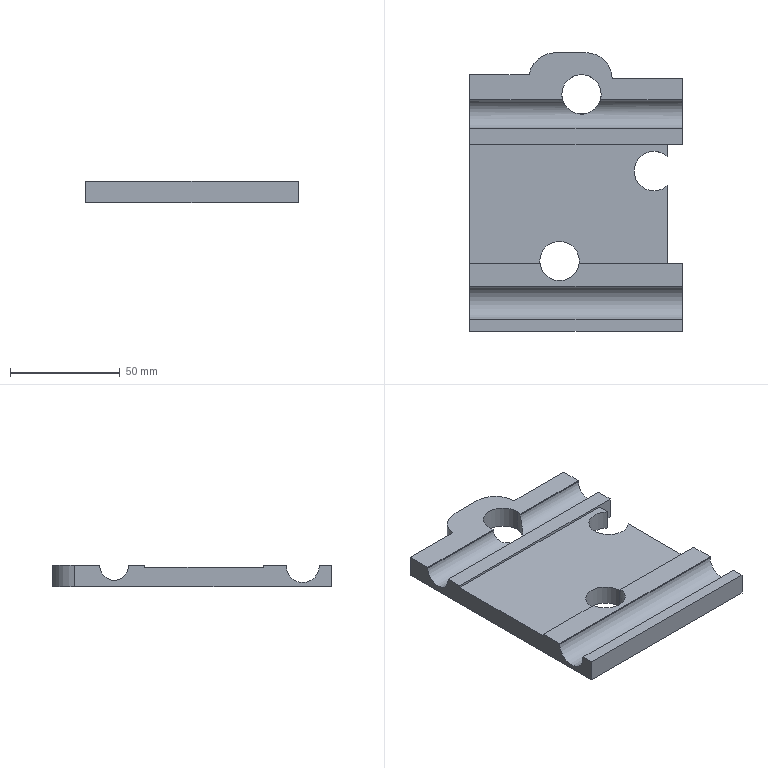Part | SolidWorks | features BaseBody 1 | 1 solid | 32 faces | box 97 x 127 x 10 mm | volume 84479 mm3 | plane 23 | cylinder 9 | commonest cylinder face diameters 18 x5 24 x2 13 x1 15 x1
STEP:
#1=CARTESIAN_POINT('',(60.,108.,10.));
#2=VERTEX_POINT('',#1);
#3=CARTESIAN_POINT('',(42.,108.,10.));
#4=VERTEX_POINT('',#3);
#5=CARTESIAN_POINT('',(51.,108.,10.));
#6=DIRECTION('',(0.,0.,1.));
#7=DIRECTION('',(1.,0.,0.));
#8=AXIS2_PLACEMENT_3D('',#5,#6,#7);
#9=CIRCLE('',#8,9.);
#10=EDGE_CURVE('',#2,#4,#9,.T.);
#11=ORIENTED_EDGE('',*,*,#10,.T.);
#12=CARTESIAN_POINT('',(42.,108.,0.));
#13=VERTEX_POINT('',#12);
#14=CARTESIAN_POINT('',(42.,108.,10.));
#15=DIRECTION('',(0.,0.,-1.));
#16=VECTOR('',#15,1000.);
#17=LINE('',#14,#16);
#18=EDGE_CURVE('',#4,#13,#17,.T.);
#19=ORIENTED_EDGE('',*,*,#18,.T.);
#20=CARTESIAN_POINT('',(60.,108.,0.));
#21=VERTEX_POINT('',#20);
#22=CARTESIAN_POINT('',(51.,108.,0.));
#23=DIRECTION('',(0.,0.,1.));
#24=DIRECTION('',(1.,0.,0.));
#25=AXIS2_PLACEMENT_3D('',#22,#23,#24);
#26=CIRCLE('',#25,9.);
#27=EDGE_CURVE('',#21,#13,#26,.T.);
#28=ORIENTED_EDGE('',*,*,#27,.F.);
#29=CARTESIAN_POINT('',(60.,108.,10.));
#30=DIRECTION('',(0.,0.,-1.));
#31=VECTOR('',#30,1000.);
#32=LINE('',#29,#31);
#33=EDGE_CURVE('',#2,#21,#32,.T.);
#34=ORIENTED_EDGE('',*,*,#33,.F.);
#35=EDGE_LOOP('',(#11,#19,#28,#34));
#36=FACE_OUTER_BOUND('',#35,.T.);
#37=CARTESIAN_POINT('',(51.,108.,10.));
#38=DIRECTION('',(0.,0.,-1.));
#39=DIRECTION('',(1.,0.,0.));
#40=AXIS2_PLACEMENT_3D('',#37,#38,#39);
#41=CYLINDRICAL_SURFACE('',#40,9.);
#42=ADVANCED_FACE('',(#36),#41,.F.);
#43=CARTESIAN_POINT('',(50.,32.,9.));
#44=VERTEX_POINT('',#43);
#45=CARTESIAN_POINT('',(32.,32.,9.));
#46=VERTEX_POINT('',#45);
#47=CARTESIAN_POINT('',(41.,32.,9.));
#48=DIRECTION('',(0.,0.,1.));
#49=DIRECTION('',(-1.,0.,0.));
#50=AXIS2_PLACEMENT_3D('',#47,#48,#49);
#51=CIRCLE('',#50,9.);
#52=EDGE_CURVE('',#44,#46,#51,.T.);
#53=ORIENTED_EDGE('',*,*,#52,.T.);
#54=CARTESIAN_POINT('',(32.,32.,0.));
#55=VERTEX_POINT('',#54);
#56=CARTESIAN_POINT('',(32.,32.,10.));
#57=DIRECTION('',(0.,0.,-1.));
#58=VECTOR('',#57,1000.);
#59=LINE('',#56,#58);
#60=EDGE_CURVE('',#46,#55,#59,.T.);
#61=ORIENTED_EDGE('',*,*,#60,.T.);
#62=CARTESIAN_POINT('',(50.,32.,0.));
#63=VERTEX_POINT('',#62);
#64=CARTESIAN_POINT('',(41.,32.,0.));
#65=DIRECTION('',(0.,0.,1.));
#66=DIRECTION('',(1.,0.,0.));
#67=AXIS2_PLACEMENT_3D('',#64,#65,#66);
#68=CIRCLE('',#67,9.);
#69=EDGE_CURVE('',#63,#55,#68,.T.);
#70=ORIENTED_EDGE('',*,*,#69,.F.);
#71=CARTESIAN_POINT('',(50.,32.,10.));
#72=DIRECTION('',(0.,0.,-1.));
#73=VECTOR('',#72,1000.);
#74=LINE('',#71,#73);
#75=EDGE_CURVE('',#44,#63,#74,.T.);
#76=ORIENTED_EDGE('',*,*,#75,.F.);
#77=EDGE_LOOP('',(#53,#61,#70,#76));
#78=FACE_OUTER_BOUND('',#77,.T.);
#79=CARTESIAN_POINT('',(41.,32.,10.));
#80=DIRECTION('',(0.,0.,-1.));
#81=DIRECTION('',(1.,0.,0.));
#82=AXIS2_PLACEMENT_3D('',#79,#80,#81);
#83=CYLINDRICAL_SURFACE('',#82,9.);
#84=ADVANCED_FACE('',(#78),#83,.F.);
#85=CARTESIAN_POINT('',(97.,5.5,9.5));
#86=VERTEX_POINT('',#85);
#87=CARTESIAN_POINT('',(0.,5.5,9.5));
#88=VERTEX_POINT('',#87);
#89=CARTESIAN_POINT('',(-27.197,5.5,9.5));
#90=DIRECTION('',(-1.,0.,0.));
#91=VECTOR('',#90,1000.);
#92=LINE('',#89,#91);
#93=EDGE_CURVE('',#86,#88,#92,.T.);
#94=ORIENTED_EDGE('',*,*,#93,.T.);
#95=CARTESIAN_POINT('',(0.,5.5,10.));
#96=VERTEX_POINT('',#95);
#97=CARTESIAN_POINT('',(0.,5.5,10.));
#98=DIRECTION('',(0.,0.,-1.));
#99=VECTOR('',#98,1000.);
#100=LINE('',#97,#99);
#101=EDGE_CURVE('',#96,#88,#100,.T.);
#102=ORIENTED_EDGE('',*,*,#101,.F.);
#103=CARTESIAN_POINT('',(97.,5.5,10.));
#104=VERTEX_POINT('',#103);
#105=CARTESIAN_POINT('',(48.5,5.5,10.));
#106=DIRECTION('',(1.,0.,0.));
#107=VECTOR('',#106,1000.);
#108=LINE('',#105,#107);
#109=EDGE_CURVE('',#96,#104,#108,.T.);
#110=ORIENTED_EDGE('',*,*,#109,.T.);
#111=CARTESIAN_POINT('',(97.,5.5,10.));
#112=DIRECTION('',(0.,0.,1.));
#113=VECTOR('',#112,1000.);
#114=LINE('',#111,#113);
#115=EDGE_CURVE('',#86,#104,#114,.T.);
#116=ORIENTED_EDGE('',*,*,#115,.F.);
#117=EDGE_LOOP('',(#94,#102,#110,#116));
#118=FACE_OUTER_BOUND('',#117,.T.);
#119=CARTESIAN_POINT('',(48.5,5.5,10.));
#120=DIRECTION('',(0.,-1.,0.));
#121=DIRECTION('',(0.,0.,-1.));
#122=AXIS2_PLACEMENT_3D('',#119,#120,#121);
#123=PLANE('',#122);
#124=ADVANCED_FACE('',(#118),#123,.F.);
#125=CARTESIAN_POINT('',(0.,20.5,10.));
#126=VERTEX_POINT('',#125);
#127=CARTESIAN_POINT('',(97.,20.5,10.));
#128=VERTEX_POINT('',#127);
#129=CARTESIAN_POINT('',(48.5,20.5,10.));
#130=DIRECTION('',(1.,0.,0.));
#131=VECTOR('',#130,1000.);
#132=LINE('',#129,#131);
#133=EDGE_CURVE('',#126,#128,#132,.T.);
#134=ORIENTED_EDGE('',*,*,#133,.F.);
#135=CARTESIAN_POINT('',(0.,20.5,9.5));
#136=VERTEX_POINT('',#135);
#137=CARTESIAN_POINT('',(0.,20.5,10.));
#138=DIRECTION('',(0.,0.,1.));
#139=VECTOR('',#138,1000.);
#140=LINE('',#137,#139);
#141=EDGE_CURVE('',#136,#126,#140,.T.);
#142=ORIENTED_EDGE('',*,*,#141,.F.);
#143=CARTESIAN_POINT('',(97.,20.5,9.5));
#144=VERTEX_POINT('',#143);
#145=CARTESIAN_POINT('',(-27.197,20.5,9.5));
#146=DIRECTION('',(-1.,0.,0.));
#147=VECTOR('',#146,1000.);
#148=LINE('',#145,#147);
#149=EDGE_CURVE('',#144,#136,#148,.T.);
#150=ORIENTED_EDGE('',*,*,#149,.F.);
#151=CARTESIAN_POINT('',(97.,20.5,10.));
#152=DIRECTION('',(0.,0.,-1.));
#153=VECTOR('',#152,1000.);
#154=LINE('',#151,#153);
#155=EDGE_CURVE('',#128,#144,#154,.T.);
#156=ORIENTED_EDGE('',*,*,#155,.F.);
#157=EDGE_LOOP('',(#134,#142,#150,#156));
#158=FACE_OUTER_BOUND('',#157,.T.);
#159=CARTESIAN_POINT('',(48.5,20.5,10.));
#160=DIRECTION('',(0.,1.,0.));
#161=DIRECTION('',(1.,0.,0.));
#162=AXIS2_PLACEMENT_3D('',#159,#160,#161);
#163=PLANE('',#162);
#164=ADVANCED_FACE('',(#158),#163,.F.);
#165=ORIENTED_EDGE('',*,*,#149,.T.);
#166=CARTESIAN_POINT('',(0.,13.,9.5));
#167=DIRECTION('',(1.,0.,0.));
#168=DIRECTION('',(0.,1.,0.));
#169=AXIS2_PLACEMENT_3D('',#166,#167,#168);
#170=CIRCLE('',#169,7.5);
#171=EDGE_CURVE('',#88,#136,#170,.T.);
#172=ORIENTED_EDGE('',*,*,#171,.F.);
#173=ORIENTED_EDGE('',*,*,#93,.F.);
#174=CARTESIAN_POINT('',(97.,13.,9.5));
#175=DIRECTION('',(-1.,0.,0.));
#176=DIRECTION('',(0.,0.,1.));
#177=AXIS2_PLACEMENT_3D('',#174,#175,#176);
#178=CIRCLE('',#177,7.5);
#179=EDGE_CURVE('',#144,#86,#178,.T.);
#180=ORIENTED_EDGE('',*,*,#179,.F.);
#181=EDGE_LOOP('',(#165,#172,#173,#180));
#182=FACE_OUTER_BOUND('',#181,.T.);
#183=CARTESIAN_POINT('',(48.5,13.,9.5));
#184=DIRECTION('',(1.,0.,0.));
#185=DIRECTION('',(0.,-1.,0.));
#186=AXIS2_PLACEMENT_3D('',#183,#184,#185);
#187=CYLINDRICAL_SURFACE('',#186,7.5);
#188=ADVANCED_FACE('',(#182),#187,.F.);
#189=CARTESIAN_POINT('',(97.,92.5,9.5));
#190=VERTEX_POINT('',#189);
#191=CARTESIAN_POINT('',(0.,92.5,9.5));
#192=VERTEX_POINT('',#191);
#193=CARTESIAN_POINT('',(-494999.993,92.5,9.5));
#194=DIRECTION('',(-1.,0.,0.));
#195=VECTOR('',#194,1000.);
#196=LINE('',#193,#195);
#197=EDGE_CURVE('',#190,#192,#196,.T.);
#198=ORIENTED_EDGE('',*,*,#197,.F.);
#199=CARTESIAN_POINT('',(97.,105.5,9.5));
#200=VERTEX_POINT('',#199);
#201=CARTESIAN_POINT('',(97.,99.,9.5));
#202=DIRECTION('',(-1.,0.,0.));
#203=DIRECTION('',(0.,0.,1.));
#204=AXIS2_PLACEMENT_3D('',#201,#202,#203);
#205=CIRCLE('',#204,6.5);
#206=EDGE_CURVE('',#200,#190,#205,.T.);
#207=ORIENTED_EDGE('',*,*,#206,.F.);
#208=CARTESIAN_POINT('',(59.646,105.5,9.5));
#209=VERTEX_POINT('',#208);
#210=CARTESIAN_POINT('',(-494999.993,105.5,9.5));
#211=DIRECTION('',(-1.,0.,0.));
#212=VECTOR('',#211,1000.);
#213=LINE('',#210,#212);
#214=EDGE_CURVE('',#200,#209,#213,.T.);
#215=ORIENTED_EDGE('',*,*,#214,.T.);
#216=CARTESIAN_POINT('',(42.354,105.5,9.5));
#217=VERTEX_POINT('',#216);
#218=CARTESIAN_POINT('',(59.646,105.5,9.5));
#219=CARTESIAN_POINT('',(59.646,105.5,8.863));
#220=CARTESIAN_POINT('',(59.621,105.408,8.242));
#221=CARTESIAN_POINT('',(59.533,105.137,7.335));
#222=CARTESIAN_POINT('',(59.495,105.024,7.039));
#223=CARTESIAN_POINT('',(59.399,104.762,6.477));
#224=CARTESIAN_POINT('',(59.34,104.613,6.207));
#225=CARTESIAN_POINT('',(59.196,104.277,5.692));
#226=CARTESIAN_POINT('',(59.109,104.09,5.446));
#227=CARTESIAN_POINT('',(58.908,103.697,4.997));
#228=CARTESIAN_POINT('',(58.793,103.49,4.792));
#229=CARTESIAN_POINT('',(58.527,103.06,4.416));
#230=CARTESIAN_POINT('',(58.375,102.835,4.245));
#231=CARTESIAN_POINT('',(58.042,102.389,3.947));
#232=CARTESIAN_POINT('',(57.86,102.167,3.818));
#233=CARTESIAN_POINT('',(57.463,101.73,3.596));
#234=CARTESIAN_POINT('',(57.247,101.514,3.502));
#235=CARTESIAN_POINT('',(56.792,101.104,3.346));
#236=CARTESIAN_POINT('',(56.552,100.91,3.284));
#237=CARTESIAN_POINT('',(56.049,100.543,3.183));
#238=CARTESIAN_POINT('',(55.783,100.37,3.144));
#239=CARTESIAN_POINT('',(55.238,100.054,3.084));
#240=CARTESIAN_POINT('',(54.958,99.911,3.063));
#241=CARTESIAN_POINT('',(54.385,99.655,3.032));
#242=CARTESIAN_POINT('',(54.091,99.541,3.022));
#243=CARTESIAN_POINT('',(53.488,99.345,3.008));
#244=CARTESIAN_POINT('',(53.182,99.263,3.005));
#245=CARTESIAN_POINT('',(52.259,99.066,2.999));
#246=CARTESIAN_POINT('',(51.634,99.,3.));
#247=CARTESIAN_POINT('',(50.685,99.,3.));
#248=CARTESIAN_POINT('',(50.367,99.017,3.));
#249=CARTESIAN_POINT('',(49.742,99.083,3.));
#250=CARTESIAN_POINT('',(49.433,99.132,3.001));
#251=CARTESIAN_POINT('',(48.82,99.262,3.005));
#252=CARTESIAN_POINT('',(48.517,99.344,3.008));
#253=CARTESIAN_POINT('',(47.917,99.539,3.022));
#254=CARTESIAN_POINT('',(47.619,99.653,3.032));
#255=CARTESIAN_POINT('',(46.758,100.038,3.078));
#256=CARTESIAN_POINT('',(46.219,100.35,3.13));
#257=CARTESIAN_POINT('',(45.465,100.897,3.28));
#258=CARTESIAN_POINT('',(45.221,101.094,3.343));
#259=CARTESIAN_POINT('',(44.764,101.504,3.498));
#260=CARTESIAN_POINT('',(44.55,101.716,3.59));
#261=CARTESIAN_POINT('',(44.153,102.152,3.81));
#262=CARTESIAN_POINT('',(43.968,102.376,3.939));
#263=CARTESIAN_POINT('',(43.631,102.825,4.238));
#264=CARTESIAN_POINT('',(43.482,103.046,4.405));
#265=CARTESIAN_POINT('',(43.216,103.476,4.778));
#266=CARTESIAN_POINT('',(43.099,103.684,4.983));
#267=CARTESIAN_POINT('',(42.895,104.082,5.436));
#268=CARTESIAN_POINT('',(42.808,104.267,5.679));
#269=CARTESIAN_POINT('',(42.663,104.604,6.192));
#270=CARTESIAN_POINT('',(42.604,104.755,6.462));
#271=CARTESIAN_POINT('',(42.506,105.021,7.031));
#272=CARTESIAN_POINT('',(42.468,105.134,7.327));
#273=CARTESIAN_POINT('',(42.409,105.315,7.927));
#274=CARTESIAN_POINT('',(42.389,105.383,8.234));
#275=CARTESIAN_POINT('',(42.361,105.476,8.862));
#276=CARTESIAN_POINT('',(42.354,105.5,9.181));
#277=CARTESIAN_POINT('',(42.354,105.5,9.5));
#278=B_SPLINE_CURVE_WITH_KNOTS('',3,(#218,#219,#220,#221,#222,#223,#224,#225,#226,#227,#228,#229,#230,#231,#232,#233,#234,#235,#236,#237,#238,#239,#240,#241,#242,#243,#244,#245,#246,#247,#248,#249,#250,#251,#252,#253,#254,#255,#256,#257,#258,#259,#260,#261,#262,#263,#264,#265,#266,#267,#268,#269,#270,#271,#272,#273,#274,#275,#276,#277),.UNSPECIFIED.,.F.,.F.,(4,2,2,2,2,2,2,2,2,2,2,2,2,2,2,2,2,2,2,2,2,2,2,2,2,2,2,2,2,4),(0.,0.001884,0.002826,0.003768,0.00471,0.005653,0.006595,0.007537,0.008479,0.009421,0.01036,0.01131,0.01225,0.01319,0.01507,0.01602,0.01696,0.0179,0.01884,0.02073,0.02167,0.02261,0.02355,0.02449,0.02544,0.02638,0.02732,0.02826,0.0292,0.03015),.UNSPECIFIED.);
#279=EDGE_CURVE('',#209,#217,#278,.T.);
#280=ORIENTED_EDGE('',*,*,#279,.T.);
#281=CARTESIAN_POINT('',(0.,105.5,9.5));
#282=VERTEX_POINT('',#281);
#283=CARTESIAN_POINT('',(-494999.993,105.5,9.5));
#284=DIRECTION('',(-1.,0.,0.));
#285=VECTOR('',#284,1000.);
#286=LINE('',#283,#285);
#287=EDGE_CURVE('',#217,#282,#286,.T.);
#288=ORIENTED_EDGE('',*,*,#287,.T.);
#289=CARTESIAN_POINT('',(0.,99.,9.5));
#290=DIRECTION('',(1.,0.,0.));
#291=DIRECTION('',(0.,1.,0.));
#292=AXIS2_PLACEMENT_3D('',#289,#290,#291);
#293=CIRCLE('',#292,6.5);
#294=EDGE_CURVE('',#192,#282,#293,.T.);
#295=ORIENTED_EDGE('',*,*,#294,.F.);
#296=EDGE_LOOP('',(#198,#207,#215,#280,#288,#295));
#297=FACE_OUTER_BOUND('',#296,.T.);
#298=CARTESIAN_POINT('',(0.,99.,9.5));
#299=DIRECTION('',(1.,0.,0.));
#300=DIRECTION('',(0.,-1.,0.));
#301=AXIS2_PLACEMENT_3D('',#298,#299,#300);
#302=CYLINDRICAL_SURFACE('',#301,6.5);
#303=ADVANCED_FACE('',(#297),#302,.F.);
#304=CARTESIAN_POINT('',(0.,92.5,10.));
#305=VERTEX_POINT('',#304);
#306=CARTESIAN_POINT('',(97.,92.5,10.));
#307=VERTEX_POINT('',#306);
#308=CARTESIAN_POINT('',(0.,92.5,10.));
#309=DIRECTION('',(1.,0.,0.));
#310=VECTOR('',#309,1000.);
#311=LINE('',#308,#310);
#312=EDGE_CURVE('',#305,#307,#311,.T.);
#313=ORIENTED_EDGE('',*,*,#312,.T.);
#314=CARTESIAN_POINT('',(97.,92.5,10.));
#315=DIRECTION('',(0.,0.,1.));
#316=VECTOR('',#315,1000.);
#317=LINE('',#314,#316);
#318=EDGE_CURVE('',#190,#307,#317,.T.);
#319=ORIENTED_EDGE('',*,*,#318,.F.);
#320=ORIENTED_EDGE('',*,*,#197,.T.);
#321=CARTESIAN_POINT('',(0.,92.5,10.));
#322=DIRECTION('',(0.,0.,-1.));
#323=VECTOR('',#322,1000.);
#324=LINE('',#321,#323);
#325=EDGE_CURVE('',#305,#192,#324,.T.);
#326=ORIENTED_EDGE('',*,*,#325,.F.);
#327=EDGE_LOOP('',(#313,#319,#320,#326));
#328=FACE_OUTER_BOUND('',#327,.T.);
#329=CARTESIAN_POINT('',(0.,92.5,10.));
#330=DIRECTION('',(0.,-1.,0.));
#331=DIRECTION('',(-1.,0.,0.));
#332=AXIS2_PLACEMENT_3D('',#329,#330,#331);
#333=PLANE('',#332);
#334=ADVANCED_FACE('',(#328),#333,.F.);
#335=CARTESIAN_POINT('',(59.646,105.5,10.));
#336=VERTEX_POINT('',#335);
#337=CARTESIAN_POINT('',(59.646,105.5,10.));
#338=DIRECTION('',(0.,0.,-1.));
#339=VECTOR('',#338,1000.);
#340=LINE('',#337,#339);
#341=EDGE_CURVE('',#336,#209,#340,.T.);
#342=ORIENTED_EDGE('',*,*,#341,.T.);
#343=ORIENTED_EDGE('',*,*,#214,.F.);
#344=CARTESIAN_POINT('',(97.,105.5,10.));
#345=VERTEX_POINT('',#344);
#346=CARTESIAN_POINT('',(97.,105.5,10.));
#347=DIRECTION('',(0.,0.,-1.));
#348=VECTOR('',#347,1000.);
#349=LINE('',#346,#348);
#350=EDGE_CURVE('',#345,#200,#349,.T.);
#351=ORIENTED_EDGE('',*,*,#350,.F.);
#352=CARTESIAN_POINT('',(0.,105.5,10.));
#353=DIRECTION('',(1.,0.,0.));
#354=VECTOR('',#353,1000.);
#355=LINE('',#352,#354);
#356=EDGE_CURVE('',#336,#345,#355,.T.);
#357=ORIENTED_EDGE('',*,*,#356,.F.);
#358=EDGE_LOOP('',(#342,#343,#351,#357));
#359=FACE_OUTER_BOUND('',#358,.T.);
#360=CARTESIAN_POINT('',(0.,105.5,10.));
#361=DIRECTION('',(0.,1.,0.));
#362=DIRECTION('',(1.,0.,0.));
#363=AXIS2_PLACEMENT_3D('',#360,#361,#362);
#364=PLANE('',#363);
#365=ADVANCED_FACE('',(#359),#364,.F.);
#366=ORIENTED_EDGE('',*,*,#287,.F.);
#367=CARTESIAN_POINT('',(42.354,105.5,10.));
#368=VERTEX_POINT('',#367);
#369=CARTESIAN_POINT('',(42.354,105.5,10.));
#370=DIRECTION('',(0.,0.,1.));
#371=VECTOR('',#370,1000.);
#372=LINE('',#369,#371);
#373=EDGE_CURVE('',#217,#368,#372,.T.);
#374=ORIENTED_EDGE('',*,*,#373,.T.);
#375=CARTESIAN_POINT('',(0.,105.5,10.));
#376=VERTEX_POINT('',#375);
#377=CARTESIAN_POINT('',(0.,105.5,10.));
#378=DIRECTION('',(1.,0.,0.));
#379=VECTOR('',#378,1000.);
#380=LINE('',#377,#379);
#381=EDGE_CURVE('',#376,#368,#380,.T.);
#382=ORIENTED_EDGE('',*,*,#381,.F.);
#383=CARTESIAN_POINT('',(0.,105.5,10.));
#384=DIRECTION('',(0.,0.,1.));
#385=VECTOR('',#384,1000.);
#386=LINE('',#383,#385);
#387=EDGE_CURVE('',#282,#376,#386,.T.);
#388=ORIENTED_EDGE('',*,*,#387,.F.);
#389=EDGE_LOOP('',(#366,#374,#382,#388));
#390=FACE_OUTER_BOUND('',#389,.T.);
#391=CARTESIAN_POINT('',(0.,105.5,10.));
#392=DIRECTION('',(0.,1.,0.));
#393=DIRECTION('',(1.,0.,0.));
#394=AXIS2_PLACEMENT_3D('',#391,#392,#393);
#395=PLANE('',#394);
#396=ADVANCED_FACE('',(#390),#395,.F.);
#397=CARTESIAN_POINT('',(90.,85.,0.));
#398=VERTEX_POINT('',#397);
#399=CARTESIAN_POINT('',(90.,85.,9.));
#400=VERTEX_POINT('',#399);
#401=CARTESIAN_POINT('',(90.,85.,-1.));
#402=DIRECTION('',(0.,0.,1.));
#403=VECTOR('',#402,1000.);
#404=LINE('',#401,#403);
#405=EDGE_CURVE('',#398,#400,#404,.T.);
#406=ORIENTED_EDGE('',*,*,#405,.T.);
#407=CARTESIAN_POINT('',(90.,79.708,9.));
#408=VERTEX_POINT('',#407);
#409=CARTESIAN_POINT('',(90.,85.,9.));
#410=DIRECTION('',(0.,-1.,0.));
#411=VECTOR('',#410,1000.);
#412=LINE('',#409,#411);
#413=EDGE_CURVE('',#400,#408,#412,.T.);
#414=ORIENTED_EDGE('',*,*,#413,.T.);
#415=CARTESIAN_POINT('',(90.,79.708,0.));
#416=VERTEX_POINT('',#415);
#417=CARTESIAN_POINT('',(90.,79.708,10.));
#418=DIRECTION('',(0.,0.,-1.));
#419=VECTOR('',#418,1000.);
#420=LINE('',#417,#419);
#421=EDGE_CURVE('',#408,#416,#420,.T.);
#422=ORIENTED_EDGE('',*,*,#421,.T.);
#423=CARTESIAN_POINT('',(90.,115.,0.));
#424=DIRECTION('',(0.,-1.,0.));
#425=VECTOR('',#424,1000.);
#426=LINE('',#423,#425);
#427=EDGE_CURVE('',#398,#416,#426,.T.);
#428=ORIENTED_EDGE('',*,*,#427,.F.);
#429=EDGE_LOOP('',(#406,#414,#422,#428));
#430=FACE_OUTER_BOUND('',#429,.T.);
#431=CARTESIAN_POINT('',(90.,85.,-1.));
#432=DIRECTION('',(-1.,0.,0.));
#433=DIRECTION('',(0.,0.,1.));
#434=AXIS2_PLACEMENT_3D('',#431,#432,#433);
#435=PLANE('',#434);
#436=ADVANCED_FACE('',(#430),#435,.F.);
#437=CARTESIAN_POINT('',(90.,66.292,0.));
#438=VERTEX_POINT('',#437);
#439=CARTESIAN_POINT('',(90.,66.292,9.));
#440=VERTEX_POINT('',#439);
#441=CARTESIAN_POINT('',(90.,66.292,10.));
#442=DIRECTION('',(0.,0.,1.));
#443=VECTOR('',#442,1000.);
#444=LINE('',#441,#443);
#445=EDGE_CURVE('',#438,#440,#444,.T.);
#446=ORIENTED_EDGE('',*,*,#445,.T.);
#447=CARTESIAN_POINT('',(90.,31.,9.));
#448=VERTEX_POINT('',#447);
#449=CARTESIAN_POINT('',(90.,85.,9.));
#450=DIRECTION('',(0.,-1.,0.));
#451=VECTOR('',#450,1000.);
#452=LINE('',#449,#451);
#453=EDGE_CURVE('',#440,#448,#452,.T.);
#454=ORIENTED_EDGE('',*,*,#453,.T.);
#455=CARTESIAN_POINT('',(90.,31.,0.));
#456=VERTEX_POINT('',#455);
#457=CARTESIAN_POINT('',(90.,31.,-1.));
#458=DIRECTION('',(0.,0.,1.));
#459=VECTOR('',#458,1000.);
#460=LINE('',#457,#459);
#461=EDGE_CURVE('',#456,#448,#460,.T.);
#462=ORIENTED_EDGE('',*,*,#461,.F.);
#463=CARTESIAN_POINT('',(90.,115.,0.));
#464=DIRECTION('',(0.,-1.,0.));
#465=VECTOR('',#464,1000.);
#466=LINE('',#463,#465);
#467=EDGE_CURVE('',#438,#456,#466,.T.);
#468=ORIENTED_EDGE('',*,*,#467,.F.);
#469=EDGE_LOOP('',(#446,#454,#462,#468));
#470=FACE_OUTER_BOUND('',#469,.T.);
#471=CARTESIAN_POINT('',(90.,85.,-1.));
#472=DIRECTION('',(-1.,0.,0.));
#473=DIRECTION('',(0.,0.,1.));
#474=AXIS2_PLACEMENT_3D('',#471,#472,#473);
#475=PLANE('',#474);
#476=ADVANCED_FACE('',(#470),#475,.F.);
#477=ORIENTED_EDGE('',*,*,#60,.F.);
#478=CARTESIAN_POINT('',(32.056,31.,9.));
#479=VERTEX_POINT('',#478);
#480=CARTESIAN_POINT('',(41.,32.,9.));
#481=DIRECTION('',(0.,0.,1.));
#482=DIRECTION('',(-1.,0.,0.));
#483=AXIS2_PLACEMENT_3D('',#480,#481,#482);
#484=CIRCLE('',#483,9.);
#485=EDGE_CURVE('',#46,#479,#484,.T.);
#486=ORIENTED_EDGE('',*,*,#485,.T.);
#487=CARTESIAN_POINT('',(32.056,31.,10.));
#488=VERTEX_POINT('',#487);
#489=CARTESIAN_POINT('',(32.056,31.,10.));
#490=DIRECTION('',(0.,0.,-1.));
#491=VECTOR('',#490,1000.);
#492=LINE('',#489,#491);
#493=EDGE_CURVE('',#488,#479,#492,.T.);
#494=ORIENTED_EDGE('',*,*,#493,.F.);
#495=CARTESIAN_POINT('',(49.944,31.,10.));
#496=VERTEX_POINT('',#495);
#497=CARTESIAN_POINT('',(41.,32.,10.));
#498=DIRECTION('',(0.,0.,1.));
#499=DIRECTION('',(1.,0.,0.));
#500=AXIS2_PLACEMENT_3D('',#497,#498,#499);
#501=CIRCLE('',#500,9.);
#502=EDGE_CURVE('',#488,#496,#501,.T.);
#503=ORIENTED_EDGE('',*,*,#502,.T.);
#504=CARTESIAN_POINT('',(49.944,31.,9.));
#505=VERTEX_POINT('',#504);
#506=CARTESIAN_POINT('',(49.944,31.,10.));
#507=DIRECTION('',(0.,0.,1.));
#508=VECTOR('',#507,1000.);
#509=LINE('',#506,#508);
#510=EDGE_CURVE('',#505,#496,#509,.T.);
#511=ORIENTED_EDGE('',*,*,#510,.F.);
#512=CARTESIAN_POINT('',(41.,32.,9.));
#513=DIRECTION('',(0.,0.,1.));
#514=DIRECTION('',(-1.,0.,0.));
#515=AXIS2_PLACEMENT_3D('',#512,#513,#514);
#516=CIRCLE('',#515,9.);
#517=EDGE_CURVE('',#505,#44,#516,.T.);
#518=ORIENTED_EDGE('',*,*,#517,.T.);
#519=ORIENTED_EDGE('',*,*,#75,.T.);
#520=CARTESIAN_POINT('',(41.,32.,0.));
#521=DIRECTION('',(0.,0.,1.));
#522=DIRECTION('',(1.,0.,0.));
#523=AXIS2_PLACEMENT_3D('',#520,#521,#522);
#524=CIRCLE('',#523,9.);
#525=EDGE_CURVE('',#55,#63,#524,.T.);
#526=ORIENTED_EDGE('',*,*,#525,.F.);
#527=EDGE_LOOP('',(#477,#486,#494,#503,#511,#518,#519,#526));
#528=FACE_OUTER_BOUND('',#527,.T.);
#529=CARTESIAN_POINT('',(41.,32.,10.));
#530=DIRECTION('',(0.,0.,-1.));
#531=DIRECTION('',(1.,0.,0.));
#532=AXIS2_PLACEMENT_3D('',#529,#530,#531);
#533=CYLINDRICAL_SURFACE('',#532,9.);
#534=ADVANCED_FACE('',(#528),#533,.F.);
#535=ORIENTED_EDGE('',*,*,#18,.F.);
#536=CARTESIAN_POINT('',(51.,108.,10.));
#537=DIRECTION('',(0.,0.,1.));
#538=DIRECTION('',(1.,0.,0.));
#539=AXIS2_PLACEMENT_3D('',#536,#537,#538);
#540=CIRCLE('',#539,9.);
#541=EDGE_CURVE('',#4,#368,#540,.T.);
#542=ORIENTED_EDGE('',*,*,#541,.T.);
#543=ORIENTED_EDGE('',*,*,#373,.F.);
#544=ORIENTED_EDGE('',*,*,#279,.F.);
#545=ORIENTED_EDGE('',*,*,#341,.F.);
#546=CARTESIAN_POINT('',(51.,108.,10.));
#547=DIRECTION('',(0.,0.,1.));
#548=DIRECTION('',(1.,0.,0.));
#549=AXIS2_PLACEMENT_3D('',#546,#547,#548);
#550=CIRCLE('',#549,9.);
#551=EDGE_CURVE('',#336,#2,#550,.T.);
#552=ORIENTED_EDGE('',*,*,#551,.T.);
#553=ORIENTED_EDGE('',*,*,#33,.T.);
#554=CARTESIAN_POINT('',(51.,108.,0.));
#555=DIRECTION('',(0.,0.,1.));
#556=DIRECTION('',(1.,0.,0.));
#557=AXIS2_PLACEMENT_3D('',#554,#555,#556);
#558=CIRCLE('',#557,9.);
#559=EDGE_CURVE('',#13,#21,#558,.T.);
#560=ORIENTED_EDGE('',*,*,#559,.F.);
#561=EDGE_LOOP('',(#535,#542,#543,#544,#545,#552,#553,#560));
#562=FACE_OUTER_BOUND('',#561,.T.);
#563=CARTESIAN_POINT('',(51.,108.,10.));
#564=DIRECTION('',(0.,0.,-1.));
#565=DIRECTION('',(1.,0.,0.));
#566=AXIS2_PLACEMENT_3D('',#563,#564,#565);
#567=CYLINDRICAL_SURFACE('',#566,9.);
#568=ADVANCED_FACE('',(#562),#567,.F.);
#569=ORIENTED_EDGE('',*,*,#421,.F.);
#570=CARTESIAN_POINT('',(84.,73.,9.));
#571=DIRECTION('',(0.,0.,1.));
#572=DIRECTION('',(-1.,0.,0.));
#573=AXIS2_PLACEMENT_3D('',#570,#571,#572);
#574=CIRCLE('',#573,9.);
#575=EDGE_CURVE('',#408,#440,#574,.T.);
#576=ORIENTED_EDGE('',*,*,#575,.T.);
#577=ORIENTED_EDGE('',*,*,#445,.F.);
#578=CARTESIAN_POINT('',(84.,73.,0.));
#579=DIRECTION('',(0.,0.,1.));
#580=DIRECTION('',(1.,0.,0.));
#581=AXIS2_PLACEMENT_3D('',#578,#579,#580);
#582=CIRCLE('',#581,9.);
#583=EDGE_CURVE('',#416,#438,#582,.T.);
#584=ORIENTED_EDGE('',*,*,#583,.F.);
#585=EDGE_LOOP('',(#569,#576,#577,#584));
#586=FACE_OUTER_BOUND('',#585,.T.);
#587=CARTESIAN_POINT('',(84.,73.,10.));
#588=DIRECTION('',(0.,0.,-1.));
#589=DIRECTION('',(1.,0.,0.));
#590=AXIS2_PLACEMENT_3D('',#587,#588,#589);
#591=CYLINDRICAL_SURFACE('',#590,9.);
#592=ADVANCED_FACE('',(#586),#591,.F.);
#593=CARTESIAN_POINT('',(0.,85.,10.));
#594=VERTEX_POINT('',#593);
#595=CARTESIAN_POINT('',(97.,85.,10.));
#596=VERTEX_POINT('',#595);
#597=CARTESIAN_POINT('',(0.,85.,10.));
#598=DIRECTION('',(1.,0.,0.));
#599=VECTOR('',#598,1000.);
#600=LINE('',#597,#599);
#601=EDGE_CURVE('',#594,#596,#600,.T.);
#602=ORIENTED_EDGE('',*,*,#601,.F.);
#603=CARTESIAN_POINT('',(0.,85.,9.));
#604=VERTEX_POINT('',#603);
#605=CARTESIAN_POINT('',(0.,85.,9.));
#606=DIRECTION('',(0.,0.,1.));
#607=VECTOR('',#606,1000.);
#608=LINE('',#605,#607);
#609=EDGE_CURVE('',#604,#594,#608,.T.);
#610=ORIENTED_EDGE('',*,*,#609,.F.);
#611=CARTESIAN_POINT('',(0.,85.,9.));
#612=DIRECTION('',(-1.,0.,0.));
#613=VECTOR('',#612,1000.);
#614=LINE('',#611,#613);
#615=EDGE_CURVE('',#400,#604,#614,.T.);
#616=ORIENTED_EDGE('',*,*,#615,.F.);
#617=ORIENTED_EDGE('',*,*,#405,.F.);
#618=CARTESIAN_POINT('',(97.,85.,0.));
#619=VERTEX_POINT('',#618);
#620=CARTESIAN_POINT('',(53.,85.,0.));
#621=DIRECTION('',(-1.,0.,0.));
#622=VECTOR('',#621,1000.);
#623=LINE('',#620,#622);
#624=EDGE_CURVE('',#619,#398,#623,.T.);
#625=ORIENTED_EDGE('',*,*,#624,.F.);
#626=CARTESIAN_POINT('',(97.,85.,9.));
#627=DIRECTION('',(0.,0.,1.));
#628=VECTOR('',#627,1000.);
#629=LINE('',#626,#628);
#630=EDGE_CURVE('',#619,#596,#629,.T.);
#631=ORIENTED_EDGE('',*,*,#630,.T.);
#632=EDGE_LOOP('',(#602,#610,#616,#617,#625,#631));
#633=FACE_OUTER_BOUND('',#632,.T.);
#634=CARTESIAN_POINT('',(0.,85.,9.));
#635=DIRECTION('',(0.,-1.,0.));
#636=DIRECTION('',(-1.,0.,0.));
#637=AXIS2_PLACEMENT_3D('',#634,#635,#636);
#638=PLANE('',#637);
#639=ADVANCED_FACE('',(#633),#638,.T.);
#640=CARTESIAN_POINT('',(97.,115.,0.));
#641=VERTEX_POINT('',#640);
#642=CARTESIAN_POINT('',(97.,0.,0.));
#643=DIRECTION('',(0.,1.,0.));
#644=VECTOR('',#643,1000.);
#645=LINE('',#642,#644);
#646=EDGE_CURVE('',#619,#641,#645,.T.);
#647=ORIENTED_EDGE('',*,*,#646,.F.);
#648=ORIENTED_EDGE('',*,*,#624,.T.);
#649=ORIENTED_EDGE('',*,*,#427,.T.);
#650=ORIENTED_EDGE('',*,*,#583,.T.);
#651=ORIENTED_EDGE('',*,*,#467,.T.);
#652=CARTESIAN_POINT('',(97.,31.,0.));
#653=VERTEX_POINT('',#652);
#654=CARTESIAN_POINT('',(53.,31.,0.));
#655=DIRECTION('',(1.,0.,0.));
#656=VECTOR('',#655,1000.);
#657=LINE('',#654,#656);
#658=EDGE_CURVE('',#456,#653,#657,.T.);
#659=ORIENTED_EDGE('',*,*,#658,.T.);
#660=CARTESIAN_POINT('',(97.,0.,0.));
#661=VERTEX_POINT('',#660);
#662=CARTESIAN_POINT('',(97.,0.,0.));
#663=DIRECTION('',(0.,1.,0.));
#664=VECTOR('',#663,1000.);
#665=LINE('',#662,#664);
#666=EDGE_CURVE('',#661,#653,#665,.T.);
#667=ORIENTED_EDGE('',*,*,#666,.F.);
#668=CARTESIAN_POINT('',(0.,0.,0.));
#669=VERTEX_POINT('',#668);
#670=CARTESIAN_POINT('',(0.,0.,0.));
#671=DIRECTION('',(1.,0.,0.));
#672=VECTOR('',#671,1000.);
#673=LINE('',#670,#672);
#674=EDGE_CURVE('',#669,#661,#673,.T.);
#675=ORIENTED_EDGE('',*,*,#674,.F.);
#676=CARTESIAN_POINT('',(0.,117.,0.));
#677=VERTEX_POINT('',#676);
#678=CARTESIAN_POINT('',(0.,117.,0.));
#679=DIRECTION('',(0.,-1.,0.));
#680=VECTOR('',#679,1000.);
#681=LINE('',#678,#680);
#682=EDGE_CURVE('',#677,#669,#681,.T.);
#683=ORIENTED_EDGE('',*,*,#682,.F.);
#684=CARTESIAN_POINT('',(27.168,117.,0.));
#685=VERTEX_POINT('',#684);
#686=CARTESIAN_POINT('',(27.168,117.,0.));
#687=DIRECTION('',(-1.,0.,0.));
#688=VECTOR('',#687,1000.);
#689=LINE('',#686,#688);
#690=EDGE_CURVE('',#685,#677,#689,.T.);
#691=ORIENTED_EDGE('',*,*,#690,.F.);
#692=CARTESIAN_POINT('',(39.,127.,0.));
#693=VERTEX_POINT('',#692);
#694=CARTESIAN_POINT('',(39.,115.,0.));
#695=DIRECTION('',(0.,0.,1.));
#696=DIRECTION('',(1.,0.,0.));
#697=AXIS2_PLACEMENT_3D('',#694,#695,#696);
#698=CIRCLE('',#697,12.);
#699=EDGE_CURVE('',#693,#685,#698,.T.);
#700=ORIENTED_EDGE('',*,*,#699,.F.);
#701=CARTESIAN_POINT('',(53.,127.,0.));
#702=VERTEX_POINT('',#701);
#703=CARTESIAN_POINT('',(53.,127.,0.));
#704=DIRECTION('',(-1.,0.,0.));
#705=VECTOR('',#704,1000.);
#706=LINE('',#703,#705);
#707=EDGE_CURVE('',#702,#693,#706,.T.);
#708=ORIENTED_EDGE('',*,*,#707,.F.);
#709=CARTESIAN_POINT('',(65.,115.,0.));
#710=VERTEX_POINT('',#709);
#711=CARTESIAN_POINT('',(53.,115.,0.));
#712=DIRECTION('',(0.,0.,1.));
#713=DIRECTION('',(1.,0.,0.));
#714=AXIS2_PLACEMENT_3D('',#711,#712,#713);
#715=CIRCLE('',#714,12.);
#716=EDGE_CURVE('',#710,#702,#715,.T.);
#717=ORIENTED_EDGE('',*,*,#716,.F.);
#718=CARTESIAN_POINT('',(97.,115.,0.));
#719=DIRECTION('',(-1.,0.,0.));
#720=VECTOR('',#719,1000.);
#721=LINE('',#718,#720);
#722=EDGE_CURVE('',#641,#710,#721,.T.);
#723=ORIENTED_EDGE('',*,*,#722,.F.);
#724=EDGE_LOOP('',(#647,#648,#649,#650,#651,#659,#667,#675,#683,#691,#700,#708,#717,#723));
#725=FACE_OUTER_BOUND('',#724,.T.);
#726=ORIENTED_EDGE('',*,*,#27,.T.);
#727=ORIENTED_EDGE('',*,*,#559,.T.);
#728=EDGE_LOOP('',(#726,#727));
#729=FACE_BOUND('',#728,.T.);
#730=ORIENTED_EDGE('',*,*,#69,.T.);
#731=ORIENTED_EDGE('',*,*,#525,.T.);
#732=EDGE_LOOP('',(#730,#731));
#733=FACE_BOUND('',#732,.T.);
#734=CARTESIAN_POINT('',(53.,115.,0.));
#735=DIRECTION('',(0.,0.,1.));
#736=DIRECTION('',(1.,0.,0.));
#737=AXIS2_PLACEMENT_3D('',#734,#735,#736);
#738=PLANE('',#737);
#739=ADVANCED_FACE('',(#725,#729,#733),#738,.F.);
#740=ORIENTED_EDGE('',*,*,#690,.T.);
#741=CARTESIAN_POINT('',(0.,117.,10.));
#742=VERTEX_POINT('',#741);
#743=CARTESIAN_POINT('',(0.,117.,10.));
#744=DIRECTION('',(0.,0.,-1.));
#745=VECTOR('',#744,1000.);
#746=LINE('',#743,#745);
#747=EDGE_CURVE('',#742,#677,#746,.T.);
#748=ORIENTED_EDGE('',*,*,#747,.F.);
#749=CARTESIAN_POINT('',(27.168,117.,10.));
#750=VERTEX_POINT('',#749);
#751=CARTESIAN_POINT('',(27.168,117.,10.));
#752=DIRECTION('',(-1.,0.,0.));
#753=VECTOR('',#752,1000.);
#754=LINE('',#751,#753);
#755=EDGE_CURVE('',#750,#742,#754,.T.);
#756=ORIENTED_EDGE('',*,*,#755,.F.);
#757=CARTESIAN_POINT('',(27.168,117.,10.));
#758=DIRECTION('',(0.,0.,-1.));
#759=VECTOR('',#758,1000.);
#760=LINE('',#757,#759);
#761=EDGE_CURVE('',#750,#685,#760,.T.);
#762=ORIENTED_EDGE('',*,*,#761,.T.);
#763=EDGE_LOOP('',(#740,#748,#756,#762));
#764=FACE_OUTER_BOUND('',#763,.T.);
#765=CARTESIAN_POINT('',(27.168,117.,10.));
#766=DIRECTION('',(0.,-1.,0.));
#767=DIRECTION('',(0.,0.,-1.));
#768=AXIS2_PLACEMENT_3D('',#765,#766,#767);
#769=PLANE('',#768);
#770=ADVANCED_FACE('',(#764),#769,.F.);
#771=ORIENTED_EDGE('',*,*,#699,.T.);
#772=ORIENTED_EDGE('',*,*,#761,.F.);
#773=CARTESIAN_POINT('',(39.,127.,10.));
#774=VERTEX_POINT('',#773);
#775=CARTESIAN_POINT('',(39.,115.,10.));
#776=DIRECTION('',(0.,0.,1.));
#777=DIRECTION('',(1.,0.,0.));
#778=AXIS2_PLACEMENT_3D('',#775,#776,#777);
#779=CIRCLE('',#778,12.);
#780=EDGE_CURVE('',#774,#750,#779,.T.);
#781=ORIENTED_EDGE('',*,*,#780,.F.);
#782=CARTESIAN_POINT('',(39.,127.,10.));
#783=DIRECTION('',(0.,0.,-1.));
#784=VECTOR('',#783,1000.);
#785=LINE('',#782,#784);
#786=EDGE_CURVE('',#774,#693,#785,.T.);
#787=ORIENTED_EDGE('',*,*,#786,.T.);
#788=EDGE_LOOP('',(#771,#772,#781,#787));
#789=FACE_OUTER_BOUND('',#788,.T.);
#790=CARTESIAN_POINT('',(39.,115.,10.));
#791=DIRECTION('',(0.,0.,-1.));
#792=DIRECTION('',(1.,0.,0.));
#793=AXIS2_PLACEMENT_3D('',#790,#791,#792);
#794=CYLINDRICAL_SURFACE('',#793,12.);
#795=ADVANCED_FACE('',(#789),#794,.T.);
#796=ORIENTED_EDGE('',*,*,#707,.T.);
#797=ORIENTED_EDGE('',*,*,#786,.F.);
#798=CARTESIAN_POINT('',(53.,127.,10.));
#799=VERTEX_POINT('',#798);
#800=CARTESIAN_POINT('',(53.,127.,10.));
#801=DIRECTION('',(-1.,0.,0.));
#802=VECTOR('',#801,1000.);
#803=LINE('',#800,#802);
#804=EDGE_CURVE('',#799,#774,#803,.T.);
#805=ORIENTED_EDGE('',*,*,#804,.F.);
#806=CARTESIAN_POINT('',(53.,127.,10.));
#807=DIRECTION('',(0.,0.,-1.));
#808=VECTOR('',#807,1000.);
#809=LINE('',#806,#808);
#810=EDGE_CURVE('',#799,#702,#809,.T.);
#811=ORIENTED_EDGE('',*,*,#810,.T.);
#812=EDGE_LOOP('',(#796,#797,#805,#811));
#813=FACE_OUTER_BOUND('',#812,.T.);
#814=CARTESIAN_POINT('',(53.,127.,10.));
#815=DIRECTION('',(0.,-1.,0.));
#816=DIRECTION('',(0.,0.,-1.));
#817=AXIS2_PLACEMENT_3D('',#814,#815,#816);
#818=PLANE('',#817);
#819=ADVANCED_FACE('',(#813),#818,.F.);
#820=ORIENTED_EDGE('',*,*,#716,.T.);
#821=ORIENTED_EDGE('',*,*,#810,.F.);
#822=CARTESIAN_POINT('',(65.,115.,10.));
#823=VERTEX_POINT('',#822);
#824=CARTESIAN_POINT('',(53.,115.,10.));
#825=DIRECTION('',(0.,0.,1.));
#826=DIRECTION('',(1.,0.,0.));
#827=AXIS2_PLACEMENT_3D('',#824,#825,#826);
#828=CIRCLE('',#827,12.);
#829=EDGE_CURVE('',#823,#799,#828,.T.);
#830=ORIENTED_EDGE('',*,*,#829,.F.);
#831=CARTESIAN_POINT('',(65.,115.,10.));
#832=DIRECTION('',(0.,0.,-1.));
#833=VECTOR('',#832,1000.);
#834=LINE('',#831,#833);
#835=EDGE_CURVE('',#823,#710,#834,.T.);
#836=ORIENTED_EDGE('',*,*,#835,.T.);
#837=EDGE_LOOP('',(#820,#821,#830,#836));
#838=FACE_OUTER_BOUND('',#837,.T.);
#839=CARTESIAN_POINT('',(53.,115.,10.));
#840=DIRECTION('',(0.,0.,-1.));
#841=DIRECTION('',(1.,0.,0.));
#842=AXIS2_PLACEMENT_3D('',#839,#840,#841);
#843=CYLINDRICAL_SURFACE('',#842,12.);
#844=ADVANCED_FACE('',(#838),#843,.T.);
#845=ORIENTED_EDGE('',*,*,#722,.T.);
#846=ORIENTED_EDGE('',*,*,#835,.F.);
#847=CARTESIAN_POINT('',(97.,115.,10.));
#848=VERTEX_POINT('',#847);
#849=CARTESIAN_POINT('',(97.,115.,10.));
#850=DIRECTION('',(-1.,0.,0.));
#851=VECTOR('',#850,1000.);
#852=LINE('',#849,#851);
#853=EDGE_CURVE('',#848,#823,#852,.T.);
#854=ORIENTED_EDGE('',*,*,#853,.F.);
#855=CARTESIAN_POINT('',(97.,115.,10.));
#856=DIRECTION('',(0.,0.,-1.));
#857=VECTOR('',#856,1000.);
#858=LINE('',#855,#857);
#859=EDGE_CURVE('',#848,#641,#858,.T.);
#860=ORIENTED_EDGE('',*,*,#859,.T.);
#861=EDGE_LOOP('',(#845,#846,#854,#860));
#862=FACE_OUTER_BOUND('',#861,.T.);
#863=CARTESIAN_POINT('',(97.,115.,10.));
#864=DIRECTION('',(0.,-1.,0.));
#865=DIRECTION('',(-1.,0.,0.));
#866=AXIS2_PLACEMENT_3D('',#863,#864,#865);
#867=PLANE('',#866);
#868=ADVANCED_FACE('',(#862),#867,.F.);
#869=CARTESIAN_POINT('',(97.,31.,10.));
#870=VERTEX_POINT('',#869);
#871=CARTESIAN_POINT('',(97.,0.,10.));
#872=DIRECTION('',(0.,1.,0.));
#873=VECTOR('',#872,1000.);
#874=LINE('',#871,#873);
#875=EDGE_CURVE('',#128,#870,#874,.T.);
#876=ORIENTED_EDGE('',*,*,#875,.F.);
#877=ORIENTED_EDGE('',*,*,#155,.T.);
#878=ORIENTED_EDGE('',*,*,#179,.T.);
#879=ORIENTED_EDGE('',*,*,#115,.T.);
#880=CARTESIAN_POINT('',(97.,0.,10.));
#881=VERTEX_POINT('',#880);
#882=CARTESIAN_POINT('',(97.,0.,10.));
#883=DIRECTION('',(0.,1.,0.));
#884=VECTOR('',#883,1000.);
#885=LINE('',#882,#884);
#886=EDGE_CURVE('',#881,#104,#885,.T.);
#887=ORIENTED_EDGE('',*,*,#886,.F.);
#888=CARTESIAN_POINT('',(97.,0.,10.));
#889=DIRECTION('',(0.,0.,-1.));
#890=VECTOR('',#889,1000.);
#891=LINE('',#888,#890);
#892=EDGE_CURVE('',#881,#661,#891,.T.);
#893=ORIENTED_EDGE('',*,*,#892,.T.);
#894=ORIENTED_EDGE('',*,*,#666,.T.);
#895=CARTESIAN_POINT('',(97.,31.,9.));
#896=DIRECTION('',(0.,0.,1.));
#897=VECTOR('',#896,1000.);
#898=LINE('',#895,#897);
#899=EDGE_CURVE('',#653,#870,#898,.T.);
#900=ORIENTED_EDGE('',*,*,#899,.T.);
#901=EDGE_LOOP('',(#876,#877,#878,#879,#887,#893,#894,#900));
#902=FACE_OUTER_BOUND('',#901,.T.);
#903=CARTESIAN_POINT('',(97.,0.,10.));
#904=DIRECTION('',(-1.,0.,0.));
#905=DIRECTION('',(0.,0.,1.));
#906=AXIS2_PLACEMENT_3D('',#903,#904,#905);
#907=PLANE('',#906);
#908=ADVANCED_FACE('',(#902),#907,.F.);
#909=ORIENTED_EDGE('',*,*,#674,.T.);
#910=ORIENTED_EDGE('',*,*,#892,.F.);
#911=CARTESIAN_POINT('',(0.,0.,10.));
#912=VERTEX_POINT('',#911);
#913=CARTESIAN_POINT('',(0.,0.,10.));
#914=DIRECTION('',(1.,0.,0.));
#915=VECTOR('',#914,1000.);
#916=LINE('',#913,#915);
#917=EDGE_CURVE('',#912,#881,#916,.T.);
#918=ORIENTED_EDGE('',*,*,#917,.F.);
#919=CARTESIAN_POINT('',(0.,0.,10.));
#920=DIRECTION('',(0.,0.,-1.));
#921=VECTOR('',#920,1000.);
#922=LINE('',#919,#921);
#923=EDGE_CURVE('',#912,#669,#922,.T.);
#924=ORIENTED_EDGE('',*,*,#923,.T.);
#925=EDGE_LOOP('',(#909,#910,#918,#924));
#926=FACE_OUTER_BOUND('',#925,.T.);
#927=CARTESIAN_POINT('',(0.,0.,10.));
#928=DIRECTION('',(0.,1.,0.));
#929=DIRECTION('',(1.,0.,0.));
#930=AXIS2_PLACEMENT_3D('',#927,#928,#929);
#931=PLANE('',#930);
#932=ADVANCED_FACE('',(#926),#931,.F.);
#933=ORIENTED_EDGE('',*,*,#171,.T.);
#934=ORIENTED_EDGE('',*,*,#141,.T.);
#935=CARTESIAN_POINT('',(0.,31.,10.));
#936=VERTEX_POINT('',#935);
#937=CARTESIAN_POINT('',(0.,117.,10.));
#938=DIRECTION('',(0.,-1.,0.));
#939=VECTOR('',#938,1000.);
#940=LINE('',#937,#939);
#941=EDGE_CURVE('',#936,#126,#940,.T.);
#942=ORIENTED_EDGE('',*,*,#941,.F.);
#943=CARTESIAN_POINT('',(0.,31.,9.));
#944=VERTEX_POINT('',#943);
#945=CARTESIAN_POINT('',(0.,31.,9.));
#946=DIRECTION('',(0.,0.,1.));
#947=VECTOR('',#946,1000.);
#948=LINE('',#945,#947);
#949=EDGE_CURVE('',#944,#936,#948,.T.);
#950=ORIENTED_EDGE('',*,*,#949,.F.);
#951=CARTESIAN_POINT('',(0.,31.,9.));
#952=DIRECTION('',(0.,1.,0.));
#953=VECTOR('',#952,1000.);
#954=LINE('',#951,#953);
#955=EDGE_CURVE('',#944,#604,#954,.T.);
#956=ORIENTED_EDGE('',*,*,#955,.T.);
#957=ORIENTED_EDGE('',*,*,#609,.T.);
#958=CARTESIAN_POINT('',(0.,117.,10.));
#959=DIRECTION('',(0.,-1.,0.));
#960=VECTOR('',#959,1000.);
#961=LINE('',#958,#960);
#962=EDGE_CURVE('',#305,#594,#961,.T.);
#963=ORIENTED_EDGE('',*,*,#962,.F.);
#964=ORIENTED_EDGE('',*,*,#325,.T.);
#965=ORIENTED_EDGE('',*,*,#294,.T.);
#966=ORIENTED_EDGE('',*,*,#387,.T.);
#967=CARTESIAN_POINT('',(0.,117.,10.));
#968=DIRECTION('',(0.,-1.,0.));
#969=VECTOR('',#968,1000.);
#970=LINE('',#967,#969);
#971=EDGE_CURVE('',#742,#376,#970,.T.);
#972=ORIENTED_EDGE('',*,*,#971,.F.);
#973=ORIENTED_EDGE('',*,*,#747,.T.);
#974=ORIENTED_EDGE('',*,*,#682,.T.);
#975=ORIENTED_EDGE('',*,*,#923,.F.);
#976=CARTESIAN_POINT('',(0.,117.,10.));
#977=DIRECTION('',(0.,-1.,0.));
#978=VECTOR('',#977,1000.);
#979=LINE('',#976,#978);
#980=EDGE_CURVE('',#96,#912,#979,.T.);
#981=ORIENTED_EDGE('',*,*,#980,.F.);
#982=ORIENTED_EDGE('',*,*,#101,.T.);
#983=EDGE_LOOP('',(#933,#934,#942,#950,#956,#957,#963,#964,#965,#966,#972,#973,#974,#975,#981,#982));
#984=FACE_OUTER_BOUND('',#983,.T.);
#985=CARTESIAN_POINT('',(0.,117.,10.));
#986=DIRECTION('',(1.,0.,0.));
#987=DIRECTION('',(0.,-1.,0.));
#988=AXIS2_PLACEMENT_3D('',#985,#986,#987);
#989=PLANE('',#988);
#990=ADVANCED_FACE('',(#984),#989,.F.);
#991=ORIENTED_EDGE('',*,*,#109,.F.);
#992=ORIENTED_EDGE('',*,*,#980,.T.);
#993=ORIENTED_EDGE('',*,*,#917,.T.);
#994=ORIENTED_EDGE('',*,*,#886,.T.);
#995=EDGE_LOOP('',(#991,#992,#993,#994));
#996=FACE_OUTER_BOUND('',#995,.T.);
#997=CARTESIAN_POINT('',(53.,115.,10.));
#998=DIRECTION('',(0.,0.,1.));
#999=DIRECTION('',(1.,0.,0.));
#1000=AXIS2_PLACEMENT_3D('',#997,#998,#999);
#1001=PLANE('',#1000);
#1002=ADVANCED_FACE('',(#996),#1001,.T.);
#1003=ORIENTED_EDGE('',*,*,#312,.F.);
#1004=ORIENTED_EDGE('',*,*,#962,.T.);
#1005=ORIENTED_EDGE('',*,*,#601,.T.);
#1006=CARTESIAN_POINT('',(97.,0.,10.));
#1007=DIRECTION('',(0.,1.,0.));
#1008=VECTOR('',#1007,1000.);
#1009=LINE('',#1006,#1008);
#1010=EDGE_CURVE('',#596,#307,#1009,.T.);
#1011=ORIENTED_EDGE('',*,*,#1010,.T.);
#1012=EDGE_LOOP('',(#1003,#1004,#1005,#1011));
#1013=FACE_OUTER_BOUND('',#1012,.T.);
#1014=CARTESIAN_POINT('',(53.,115.,10.));
#1015=DIRECTION('',(0.,0.,1.));
#1016=DIRECTION('',(1.,0.,0.));
#1017=AXIS2_PLACEMENT_3D('',#1014,#1015,#1016);
#1018=PLANE('',#1017);
#1019=ADVANCED_FACE('',(#1013),#1018,.T.);
#1020=CARTESIAN_POINT('',(97.,31.,10.));
#1021=DIRECTION('',(-1.,0.,0.));
#1022=VECTOR('',#1021,1000.);
#1023=LINE('',#1020,#1022);
#1024=EDGE_CURVE('',#488,#936,#1023,.T.);
#1025=ORIENTED_EDGE('',*,*,#1024,.F.);
#1026=ORIENTED_EDGE('',*,*,#493,.T.);
#1027=CARTESIAN_POINT('',(97.,31.,9.));
#1028=DIRECTION('',(1.,0.,0.));
#1029=VECTOR('',#1028,1000.);
#1030=LINE('',#1027,#1029);
#1031=EDGE_CURVE('',#944,#479,#1030,.T.);
#1032=ORIENTED_EDGE('',*,*,#1031,.F.);
#1033=ORIENTED_EDGE('',*,*,#949,.T.);
#1034=EDGE_LOOP('',(#1025,#1026,#1032,#1033));
#1035=FACE_OUTER_BOUND('',#1034,.T.);
#1036=CARTESIAN_POINT('',(97.,31.,9.));
#1037=DIRECTION('',(0.,1.,0.));
#1038=DIRECTION('',(1.,0.,0.));
#1039=AXIS2_PLACEMENT_3D('',#1036,#1037,#1038);
#1040=PLANE('',#1039);
#1041=ADVANCED_FACE('',(#1035),#1040,.T.);
#1042=CARTESIAN_POINT('',(97.,31.,9.));
#1043=DIRECTION('',(1.,0.,0.));
#1044=VECTOR('',#1043,1000.);
#1045=LINE('',#1042,#1044);
#1046=EDGE_CURVE('',#505,#448,#1045,.T.);
#1047=ORIENTED_EDGE('',*,*,#1046,.F.);
#1048=ORIENTED_EDGE('',*,*,#510,.T.);
#1049=CARTESIAN_POINT('',(97.,31.,10.));
#1050=DIRECTION('',(-1.,0.,0.));
#1051=VECTOR('',#1050,1000.);
#1052=LINE('',#1049,#1051);
#1053=EDGE_CURVE('',#870,#496,#1052,.T.);
#1054=ORIENTED_EDGE('',*,*,#1053,.F.);
#1055=ORIENTED_EDGE('',*,*,#899,.F.);
#1056=ORIENTED_EDGE('',*,*,#658,.F.);
#1057=ORIENTED_EDGE('',*,*,#461,.T.);
#1058=EDGE_LOOP('',(#1047,#1048,#1054,#1055,#1056,#1057));
#1059=FACE_OUTER_BOUND('',#1058,.T.);
#1060=CARTESIAN_POINT('',(97.,31.,9.));
#1061=DIRECTION('',(0.,1.,0.));
#1062=DIRECTION('',(1.,0.,0.));
#1063=AXIS2_PLACEMENT_3D('',#1060,#1061,#1062);
#1064=PLANE('',#1063);
#1065=ADVANCED_FACE('',(#1059),#1064,.T.);
#1066=ORIENTED_EDGE('',*,*,#413,.F.);
#1067=ORIENTED_EDGE('',*,*,#615,.T.);
#1068=ORIENTED_EDGE('',*,*,#955,.F.);
#1069=ORIENTED_EDGE('',*,*,#1031,.T.);
#1070=ORIENTED_EDGE('',*,*,#485,.F.);
#1071=ORIENTED_EDGE('',*,*,#52,.F.);
#1072=ORIENTED_EDGE('',*,*,#517,.F.);
#1073=ORIENTED_EDGE('',*,*,#1046,.T.);
#1074=ORIENTED_EDGE('',*,*,#453,.F.);
#1075=ORIENTED_EDGE('',*,*,#575,.F.);
#1076=EDGE_LOOP('',(#1066,#1067,#1068,#1069,#1070,#1071,#1072,#1073,#1074,#1075));
#1077=FACE_OUTER_BOUND('',#1076,.T.);
#1078=CARTESIAN_POINT('',(0.,0.,9.));
#1079=DIRECTION('',(0.,0.,-1.));
#1080=DIRECTION('',(0.,-1.,0.));
#1081=AXIS2_PLACEMENT_3D('',#1078,#1079,#1080);
#1082=PLANE('',#1081);
#1083=ADVANCED_FACE('',(#1077),#1082,.F.);
#1084=CARTESIAN_POINT('',(97.,0.,10.));
#1085=DIRECTION('',(0.,1.,0.));
#1086=VECTOR('',#1085,1000.);
#1087=LINE('',#1084,#1086);
#1088=EDGE_CURVE('',#345,#848,#1087,.T.);
#1089=ORIENTED_EDGE('',*,*,#1088,.F.);
#1090=ORIENTED_EDGE('',*,*,#350,.T.);
#1091=ORIENTED_EDGE('',*,*,#206,.T.);
#1092=ORIENTED_EDGE('',*,*,#318,.T.);
#1093=ORIENTED_EDGE('',*,*,#1010,.F.);
#1094=ORIENTED_EDGE('',*,*,#630,.F.);
#1095=ORIENTED_EDGE('',*,*,#646,.T.);
#1096=ORIENTED_EDGE('',*,*,#859,.F.);
#1097=EDGE_LOOP('',(#1089,#1090,#1091,#1092,#1093,#1094,#1095,#1096));
#1098=FACE_OUTER_BOUND('',#1097,.T.);
#1099=CARTESIAN_POINT('',(97.,0.,10.));
#1100=DIRECTION('',(-1.,0.,0.));
#1101=DIRECTION('',(0.,0.,1.));
#1102=AXIS2_PLACEMENT_3D('',#1099,#1100,#1101);
#1103=PLANE('',#1102);
#1104=ADVANCED_FACE('',(#1098),#1103,.F.);
#1105=ORIENTED_EDGE('',*,*,#971,.T.);
#1106=ORIENTED_EDGE('',*,*,#381,.T.);
#1107=ORIENTED_EDGE('',*,*,#541,.F.);
#1108=ORIENTED_EDGE('',*,*,#10,.F.);
#1109=ORIENTED_EDGE('',*,*,#551,.F.);
#1110=ORIENTED_EDGE('',*,*,#356,.T.);
#1111=ORIENTED_EDGE('',*,*,#1088,.T.);
#1112=ORIENTED_EDGE('',*,*,#853,.T.);
#1113=ORIENTED_EDGE('',*,*,#829,.T.);
#1114=ORIENTED_EDGE('',*,*,#804,.T.);
#1115=ORIENTED_EDGE('',*,*,#780,.T.);
#1116=ORIENTED_EDGE('',*,*,#755,.T.);
#1117=EDGE_LOOP('',(#1105,#1106,#1107,#1108,#1109,#1110,#1111,#1112,#1113,#1114,#1115,#1116));
#1118=FACE_OUTER_BOUND('',#1117,.T.);
#1119=CARTESIAN_POINT('',(53.,115.,10.));
#1120=DIRECTION('',(0.,0.,1.));
#1121=DIRECTION('',(1.,0.,0.));
#1122=AXIS2_PLACEMENT_3D('',#1119,#1120,#1121);
#1123=PLANE('',#1122);
#1124=ADVANCED_FACE('',(#1118),#1123,.T.);
#1125=ORIENTED_EDGE('',*,*,#941,.T.);
#1126=ORIENTED_EDGE('',*,*,#133,.T.);
#1127=ORIENTED_EDGE('',*,*,#875,.T.);
#1128=ORIENTED_EDGE('',*,*,#1053,.T.);
#1129=ORIENTED_EDGE('',*,*,#502,.F.);
#1130=ORIENTED_EDGE('',*,*,#1024,.T.);
#1131=EDGE_LOOP('',(#1125,#1126,#1127,#1128,#1129,#1130));
#1132=FACE_OUTER_BOUND('',#1131,.T.);
#1133=CARTESIAN_POINT('',(53.,115.,10.));
#1134=DIRECTION('',(0.,0.,1.));
#1135=DIRECTION('',(1.,0.,0.));
#1136=AXIS2_PLACEMENT_3D('',#1133,#1134,#1135);
#1137=PLANE('',#1136);
#1138=ADVANCED_FACE('',(#1132),#1137,.T.);
#1139=CLOSED_SHELL('',(#42,#84,#124,#164,#188,#303,#334,#365,#396,#436,#476,#534,#568,#592,#639,#739,#770,#795,#819,#844,#868,#908,#932,#990,#1002,#1019,#1041,#1065,#1083,#1104,#1124,#1138));
#1140=MANIFOLD_SOLID_BREP('',#1139);
#1141=CARTESIAN_POINT('',(0.,0.,0.));
#1142=DIRECTION('',(0.,0.,1.));
#1143=DIRECTION('',(1.,0.,0.));
#1144=AXIS2_PLACEMENT_3D('',#1141,#1142,#1143);
#1145=(LENGTH_UNIT()NAMED_UNIT(*)SI_UNIT(.MILLI.,.METRE.));
#1146=UNCERTAINTY_MEASURE_WITH_UNIT(LENGTH_MEASURE(0.00001),#1145,'','');
#1147=(NAMED_UNIT(*)PLANE_ANGLE_UNIT()SI_UNIT($,.RADIAN.));
#1148=(NAMED_UNIT(*)SI_UNIT($,.STERADIAN.)SOLID_ANGLE_UNIT());
#1149=(GEOMETRIC_REPRESENTATION_CONTEXT(3)GLOBAL_UNCERTAINTY_ASSIGNED_CONTEXT((#1146))GLOBAL_UNIT_ASSIGNED_CONTEXT((#1145,#1147,#1148))REPRESENTATION_CONTEXT('',''));
#1150=ADVANCED_BREP_SHAPE_REPRESENTATION('',(#1140,#1144),#1149);